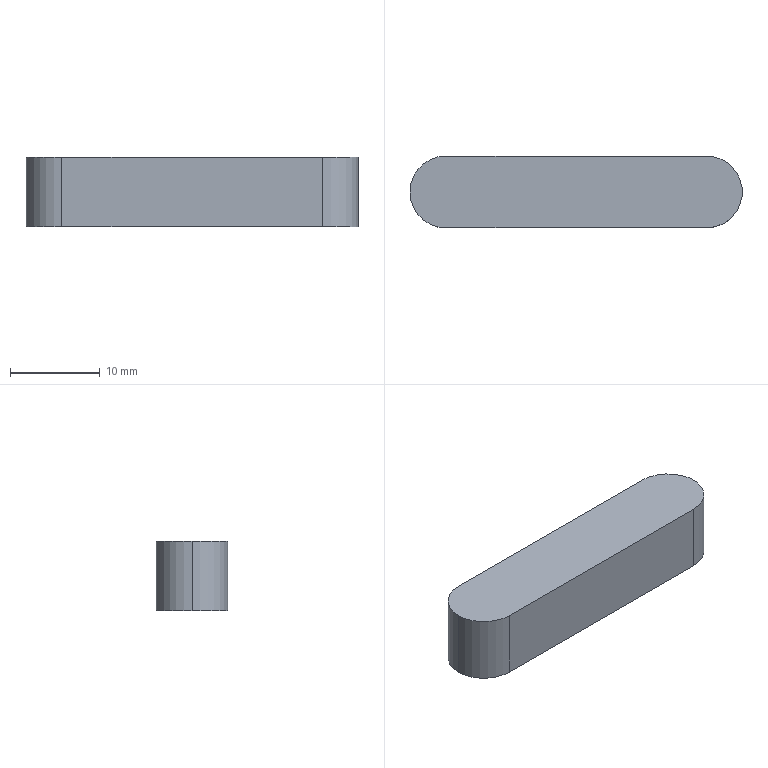Part | STEP file | Keyway 8x38V11_Default<Machined> | 1 solid | 7 faces | box 37 x 8 x 7.7 mm | volume 2173 mm3 | plane 4 | cylinder 3 | commonest cylinder face diameters 8 x3
STEP:
#1=CARTESIAN_POINT('',(0.,0.,0.));
#2=DIRECTION('',(0.,0.,1.));
#3=DIRECTION('',(1.,0.,0.));
#4=AXIS2_PLACEMENT_3D('',#1,#2,#3);
#5=CARTESIAN_POINT('',(-33.,0.,7.7));
#6=VERTEX_POINT('',#5);
#7=CARTESIAN_POINT('',(-29.,-4.,7.7));
#8=VERTEX_POINT('',#7);
#9=CARTESIAN_POINT('',(-29.,0.,7.7));
#10=DIRECTION('',(0.,0.,1.));
#11=DIRECTION('',(1.,0.,0.));
#12=AXIS2_PLACEMENT_3D('',#9,#10,#11);
#13=CIRCLE('',#12,4.);
#14=CARTESIAN_POINT('',(-29.,0.,7.7));
#15=DIRECTION('',(0.,0.,-1.));
#16=DIRECTION('',(-1.,0.,0.));
#17=AXIS2_PLACEMENT_3D('',#14,#15,#16);
#18=CYLINDRICAL_SURFACE('',#17,4.);
#19=CARTESIAN_POINT('',(9.425,0.));
#20=DIRECTION('',(-1.,0.));
#21=VECTOR('',#20,1.);
#22=LINE('',#19,#21);
#23=(GEOMETRIC_REPRESENTATION_CONTEXT(2)PARAMETRIC_REPRESENTATION_CONTEXT()REPRESENTATION_CONTEXT('',''));
#24=DEFINITIONAL_REPRESENTATION('',(#22),#23);
#25=PCURVE('',#18,#24);
#26=CARTESIAN_POINT('',(0.,0.,7.7));
#27=DIRECTION('',(0.,0.,1.));
#28=DIRECTION('',(1.,0.,0.));
#29=AXIS2_PLACEMENT_3D('',#26,#27,#28);
#30=PLANE('',#29);
#31=CARTESIAN_POINT('',(-29.,0.));
#32=DIRECTION('',(1.,0.));
#33=AXIS2_PLACEMENT_2D('',#31,#32);
#34=CIRCLE('',#33,4.);
#35=(GEOMETRIC_REPRESENTATION_CONTEXT(2)PARAMETRIC_REPRESENTATION_CONTEXT()REPRESENTATION_CONTEXT('',''));
#36=DEFINITIONAL_REPRESENTATION('',(#34),#35);
#37=PCURVE('',#30,#36);
#38=SURFACE_CURVE('',#13,(#25,#37),.PCURVE_S1.);
#39=EDGE_CURVE('',#6,#8,#38,.T.);
#40=ORIENTED_EDGE('',*,*,#39,.F.);
#41=CARTESIAN_POINT('',(-33.,0.,0.));
#42=VERTEX_POINT('',#41);
#43=CARTESIAN_POINT('',(-33.,0.,7.7));
#44=DIRECTION('',(0.,0.,-1.));
#45=VECTOR('',#44,1.);
#46=LINE('',#43,#45);
#47=CARTESIAN_POINT('',(6.283,0.));
#48=DIRECTION('',(0.,1.));
#49=VECTOR('',#48,1.);
#50=LINE('',#47,#49);
#51=(GEOMETRIC_REPRESENTATION_CONTEXT(2)PARAMETRIC_REPRESENTATION_CONTEXT()REPRESENTATION_CONTEXT('',''));
#52=DEFINITIONAL_REPRESENTATION('',(#50),#51);
#53=PCURVE('',#18,#52);
#54=CARTESIAN_POINT('',(-29.,0.,7.7));
#55=DIRECTION('',(0.,0.,-1.));
#56=DIRECTION('',(-1.,0.,0.));
#57=AXIS2_PLACEMENT_3D('',#54,#55,#56);
#58=CYLINDRICAL_SURFACE('',#57,4.);
#59=CARTESIAN_POINT('',(0.,0.));
#60=DIRECTION('',(0.,1.));
#61=VECTOR('',#60,1.);
#62=LINE('',#59,#61);
#63=(GEOMETRIC_REPRESENTATION_CONTEXT(2)PARAMETRIC_REPRESENTATION_CONTEXT()REPRESENTATION_CONTEXT('',''));
#64=DEFINITIONAL_REPRESENTATION('',(#62),#63);
#65=PCURVE('',#58,#64);
#66=SURFACE_CURVE('',#46,(#53,#65),.PCURVE_S1.);
#67=EDGE_CURVE('',#6,#42,#66,.T.);
#68=ORIENTED_EDGE('',*,*,#67,.T.);
#69=CARTESIAN_POINT('',(-29.,-4.,0.));
#70=VERTEX_POINT('',#69);
#71=CARTESIAN_POINT('',(-29.,0.,0.));
#72=DIRECTION('',(0.,0.,1.));
#73=DIRECTION('',(1.,0.,0.));
#74=AXIS2_PLACEMENT_3D('',#71,#72,#73);
#75=CIRCLE('',#74,4.);
#76=CARTESIAN_POINT('',(9.425,7.7));
#77=DIRECTION('',(-1.,0.));
#78=VECTOR('',#77,1.);
#79=LINE('',#76,#78);
#80=(GEOMETRIC_REPRESENTATION_CONTEXT(2)PARAMETRIC_REPRESENTATION_CONTEXT()REPRESENTATION_CONTEXT('',''));
#81=DEFINITIONAL_REPRESENTATION('',(#79),#80);
#82=PCURVE('',#18,#81);
#83=CARTESIAN_POINT('',(0.,0.,0.));
#84=DIRECTION('',(0.,0.,1.));
#85=DIRECTION('',(1.,0.,0.));
#86=AXIS2_PLACEMENT_3D('',#83,#84,#85);
#87=PLANE('',#86);
#88=CARTESIAN_POINT('',(-29.,0.));
#89=DIRECTION('',(1.,0.));
#90=AXIS2_PLACEMENT_2D('',#88,#89);
#91=CIRCLE('',#90,4.);
#92=(GEOMETRIC_REPRESENTATION_CONTEXT(2)PARAMETRIC_REPRESENTATION_CONTEXT()REPRESENTATION_CONTEXT('',''));
#93=DEFINITIONAL_REPRESENTATION('',(#91),#92);
#94=PCURVE('',#87,#93);
#95=SURFACE_CURVE('',#75,(#82,#94),.PCURVE_S1.);
#96=EDGE_CURVE('',#42,#70,#95,.T.);
#97=ORIENTED_EDGE('',*,*,#96,.T.);
#98=CARTESIAN_POINT('',(-29.,-4.,7.7));
#99=DIRECTION('',(0.,0.,-1.));
#100=VECTOR('',#99,1.);
#101=LINE('',#98,#100);
#102=CARTESIAN_POINT('',(4.712,0.));
#103=DIRECTION('',(0.,1.));
#104=VECTOR('',#103,1.);
#105=LINE('',#102,#104);
#106=(GEOMETRIC_REPRESENTATION_CONTEXT(2)PARAMETRIC_REPRESENTATION_CONTEXT()REPRESENTATION_CONTEXT('',''));
#107=DEFINITIONAL_REPRESENTATION('',(#105),#106);
#108=PCURVE('',#18,#107);
#109=CARTESIAN_POINT('',(0.,-4.,7.7));
#110=DIRECTION('',(0.,1.,0.));
#111=DIRECTION('',(-1.,0.,0.));
#112=AXIS2_PLACEMENT_3D('',#109,#110,#111);
#113=PLANE('',#112);
#114=CARTESIAN_POINT('',(29.,0.));
#115=DIRECTION('',(0.,-1.));
#116=VECTOR('',#115,1.);
#117=LINE('',#114,#116);
#118=(GEOMETRIC_REPRESENTATION_CONTEXT(2)PARAMETRIC_REPRESENTATION_CONTEXT()REPRESENTATION_CONTEXT('',''));
#119=DEFINITIONAL_REPRESENTATION('',(#117),#118);
#120=PCURVE('',#113,#119);
#121=SURFACE_CURVE('',#101,(#108,#120),.PCURVE_S1.);
#122=EDGE_CURVE('',#8,#70,#121,.T.);
#123=ORIENTED_EDGE('',*,*,#122,.F.);
#124=EDGE_LOOP('',(#40,#68,#97,#123));
#125=FACE_BOUND('',#124,.T.);
#126=ADVANCED_FACE('',(#125),#18,.T.);
#127=CARTESIAN_POINT('',(0.,-4.,0.));
#128=VERTEX_POINT('',#127);
#129=CARTESIAN_POINT('',(0.,4.,0.));
#130=VERTEX_POINT('',#129);
#131=CARTESIAN_POINT('',(0.,0.,0.));
#132=DIRECTION('',(0.,0.,1.));
#133=DIRECTION('',(1.,0.,0.));
#134=AXIS2_PLACEMENT_3D('',#131,#132,#133);
#135=CIRCLE('',#134,4.);
#136=CARTESIAN_POINT('',(0.,0.,7.7));
#137=DIRECTION('',(0.,0.,-1.));
#138=DIRECTION('',(-1.,0.,0.));
#139=AXIS2_PLACEMENT_3D('',#136,#137,#138);
#140=CYLINDRICAL_SURFACE('',#139,4.);
#141=CARTESIAN_POINT('',(9.425,7.7));
#142=DIRECTION('',(-1.,0.));
#143=VECTOR('',#142,1.);
#144=LINE('',#141,#143);
#145=(GEOMETRIC_REPRESENTATION_CONTEXT(2)PARAMETRIC_REPRESENTATION_CONTEXT()REPRESENTATION_CONTEXT('',''));
#146=DEFINITIONAL_REPRESENTATION('',(#144),#145);
#147=PCURVE('',#140,#146);
#148=CARTESIAN_POINT('',(0.,0.));
#149=DIRECTION('',(1.,0.));
#150=AXIS2_PLACEMENT_2D('',#148,#149);
#151=CIRCLE('',#150,4.);
#152=(GEOMETRIC_REPRESENTATION_CONTEXT(2)PARAMETRIC_REPRESENTATION_CONTEXT()REPRESENTATION_CONTEXT('',''));
#153=DEFINITIONAL_REPRESENTATION('',(#151),#152);
#154=PCURVE('',#87,#153);
#155=SURFACE_CURVE('',#135,(#147,#154),.PCURVE_S1.);
#156=EDGE_CURVE('',#128,#130,#155,.T.);
#157=ORIENTED_EDGE('',*,*,#156,.T.);
#158=CARTESIAN_POINT('',(0.,4.,7.7));
#159=VERTEX_POINT('',#158);
#160=CARTESIAN_POINT('',(0.,4.,7.7));
#161=DIRECTION('',(0.,0.,-1.));
#162=VECTOR('',#161,1.);
#163=LINE('',#160,#162);
#164=CARTESIAN_POINT('',(1.571,0.));
#165=DIRECTION('',(0.,1.));
#166=VECTOR('',#165,1.);
#167=LINE('',#164,#166);
#168=(GEOMETRIC_REPRESENTATION_CONTEXT(2)PARAMETRIC_REPRESENTATION_CONTEXT()REPRESENTATION_CONTEXT('',''));
#169=DEFINITIONAL_REPRESENTATION('',(#167),#168);
#170=PCURVE('',#140,#169);
#171=CARTESIAN_POINT('',(0.,4.,7.7));
#172=DIRECTION('',(0.,-1.,0.));
#173=DIRECTION('',(1.,0.,0.));
#174=AXIS2_PLACEMENT_3D('',#171,#172,#173);
#175=PLANE('',#174);
#176=CARTESIAN_POINT('',(0.,0.));
#177=DIRECTION('',(0.,-1.));
#178=VECTOR('',#177,1.);
#179=LINE('',#176,#178);
#180=(GEOMETRIC_REPRESENTATION_CONTEXT(2)PARAMETRIC_REPRESENTATION_CONTEXT()REPRESENTATION_CONTEXT('',''));
#181=DEFINITIONAL_REPRESENTATION('',(#179),#180);
#182=PCURVE('',#175,#181);
#183=SURFACE_CURVE('',#163,(#170,#182),.PCURVE_S1.);
#184=EDGE_CURVE('',#159,#130,#183,.T.);
#185=ORIENTED_EDGE('',*,*,#184,.F.);
#186=CARTESIAN_POINT('',(0.,-4.,7.7));
#187=VERTEX_POINT('',#186);
#188=CARTESIAN_POINT('',(0.,0.,7.7));
#189=DIRECTION('',(0.,0.,1.));
#190=DIRECTION('',(1.,0.,0.));
#191=AXIS2_PLACEMENT_3D('',#188,#189,#190);
#192=CIRCLE('',#191,4.);
#193=CARTESIAN_POINT('',(9.425,0.));
#194=DIRECTION('',(-1.,0.));
#195=VECTOR('',#194,1.);
#196=LINE('',#193,#195);
#197=(GEOMETRIC_REPRESENTATION_CONTEXT(2)PARAMETRIC_REPRESENTATION_CONTEXT()REPRESENTATION_CONTEXT('',''));
#198=DEFINITIONAL_REPRESENTATION('',(#196),#197);
#199=PCURVE('',#140,#198);
#200=CARTESIAN_POINT('',(0.,0.));
#201=DIRECTION('',(1.,0.));
#202=AXIS2_PLACEMENT_2D('',#200,#201);
#203=CIRCLE('',#202,4.);
#204=(GEOMETRIC_REPRESENTATION_CONTEXT(2)PARAMETRIC_REPRESENTATION_CONTEXT()REPRESENTATION_CONTEXT('',''));
#205=DEFINITIONAL_REPRESENTATION('',(#203),#204);
#206=PCURVE('',#30,#205);
#207=SURFACE_CURVE('',#192,(#199,#206),.PCURVE_S1.);
#208=EDGE_CURVE('',#187,#159,#207,.T.);
#209=ORIENTED_EDGE('',*,*,#208,.F.);
#210=CARTESIAN_POINT('',(0.,-4.,7.7));
#211=DIRECTION('',(0.,0.,-1.));
#212=VECTOR('',#211,1.);
#213=LINE('',#210,#212);
#214=CARTESIAN_POINT('',(4.712,0.));
#215=DIRECTION('',(0.,1.));
#216=VECTOR('',#215,1.);
#217=LINE('',#214,#216);
#218=(GEOMETRIC_REPRESENTATION_CONTEXT(2)PARAMETRIC_REPRESENTATION_CONTEXT()REPRESENTATION_CONTEXT('',''));
#219=DEFINITIONAL_REPRESENTATION('',(#217),#218);
#220=PCURVE('',#140,#219);
#221=CARTESIAN_POINT('',(0.,0.));
#222=DIRECTION('',(0.,-1.));
#223=VECTOR('',#222,1.);
#224=LINE('',#221,#223);
#225=(GEOMETRIC_REPRESENTATION_CONTEXT(2)PARAMETRIC_REPRESENTATION_CONTEXT()REPRESENTATION_CONTEXT('',''));
#226=DEFINITIONAL_REPRESENTATION('',(#224),#225);
#227=PCURVE('',#113,#226);
#228=SURFACE_CURVE('',#213,(#220,#227),.PCURVE_S1.);
#229=EDGE_CURVE('',#187,#128,#228,.T.);
#230=ORIENTED_EDGE('',*,*,#229,.T.);
#231=EDGE_LOOP('',(#157,#185,#209,#230));
#232=FACE_BOUND('',#231,.T.);
#233=ADVANCED_FACE('',(#232),#140,.T.);
#234=CARTESIAN_POINT('',(-29.,4.,0.));
#235=VERTEX_POINT('',#234);
#236=CARTESIAN_POINT('',(0.,4.,0.));
#237=DIRECTION('',(-1.,0.,0.));
#238=VECTOR('',#237,1.);
#239=LINE('',#236,#238);
#240=CARTESIAN_POINT('',(0.,-7.7));
#241=DIRECTION('',(-1.,0.));
#242=VECTOR('',#241,1.);
#243=LINE('',#240,#242);
#244=(GEOMETRIC_REPRESENTATION_CONTEXT(2)PARAMETRIC_REPRESENTATION_CONTEXT()REPRESENTATION_CONTEXT('',''));
#245=DEFINITIONAL_REPRESENTATION('',(#243),#244);
#246=PCURVE('',#175,#245);
#247=CARTESIAN_POINT('',(0.,4.));
#248=DIRECTION('',(-1.,0.));
#249=VECTOR('',#248,1.);
#250=LINE('',#247,#249);
#251=(GEOMETRIC_REPRESENTATION_CONTEXT(2)PARAMETRIC_REPRESENTATION_CONTEXT()REPRESENTATION_CONTEXT('',''));
#252=DEFINITIONAL_REPRESENTATION('',(#250),#251);
#253=PCURVE('',#87,#252);
#254=SURFACE_CURVE('',#239,(#246,#253),.PCURVE_S1.);
#255=EDGE_CURVE('',#130,#235,#254,.T.);
#256=ORIENTED_EDGE('',*,*,#255,.T.);
#257=CARTESIAN_POINT('',(-29.,4.,7.7));
#258=VERTEX_POINT('',#257);
#259=CARTESIAN_POINT('',(-29.,4.,7.7));
#260=DIRECTION('',(0.,0.,-1.));
#261=VECTOR('',#260,1.);
#262=LINE('',#259,#261);
#263=CARTESIAN_POINT('',(-29.,0.));
#264=DIRECTION('',(0.,-1.));
#265=VECTOR('',#264,1.);
#266=LINE('',#263,#265);
#267=(GEOMETRIC_REPRESENTATION_CONTEXT(2)PARAMETRIC_REPRESENTATION_CONTEXT()REPRESENTATION_CONTEXT('',''));
#268=DEFINITIONAL_REPRESENTATION('',(#266),#267);
#269=PCURVE('',#175,#268);
#270=CARTESIAN_POINT('',(1.571,0.));
#271=DIRECTION('',(0.,1.));
#272=VECTOR('',#271,1.);
#273=LINE('',#270,#272);
#274=(GEOMETRIC_REPRESENTATION_CONTEXT(2)PARAMETRIC_REPRESENTATION_CONTEXT()REPRESENTATION_CONTEXT('',''));
#275=DEFINITIONAL_REPRESENTATION('',(#273),#274);
#276=PCURVE('',#58,#275);
#277=SURFACE_CURVE('',#262,(#269,#276),.PCURVE_S1.);
#278=EDGE_CURVE('',#258,#235,#277,.T.);
#279=ORIENTED_EDGE('',*,*,#278,.F.);
#280=CARTESIAN_POINT('',(0.,4.,7.7));
#281=DIRECTION('',(-1.,0.,0.));
#282=VECTOR('',#281,1.);
#283=LINE('',#280,#282);
#284=CARTESIAN_POINT('',(0.,0.));
#285=DIRECTION('',(-1.,0.));
#286=VECTOR('',#285,1.);
#287=LINE('',#284,#286);
#288=(GEOMETRIC_REPRESENTATION_CONTEXT(2)PARAMETRIC_REPRESENTATION_CONTEXT()REPRESENTATION_CONTEXT('',''));
#289=DEFINITIONAL_REPRESENTATION('',(#287),#288);
#290=PCURVE('',#175,#289);
#291=CARTESIAN_POINT('',(0.,4.));
#292=DIRECTION('',(-1.,0.));
#293=VECTOR('',#292,1.);
#294=LINE('',#291,#293);
#295=(GEOMETRIC_REPRESENTATION_CONTEXT(2)PARAMETRIC_REPRESENTATION_CONTEXT()REPRESENTATION_CONTEXT('',''));
#296=DEFINITIONAL_REPRESENTATION('',(#294),#295);
#297=PCURVE('',#30,#296);
#298=SURFACE_CURVE('',#283,(#290,#297),.PCURVE_S1.);
#299=EDGE_CURVE('',#159,#258,#298,.T.);
#300=ORIENTED_EDGE('',*,*,#299,.F.);
#301=ORIENTED_EDGE('',*,*,#184,.T.);
#302=EDGE_LOOP('',(#256,#279,#300,#301));
#303=FACE_BOUND('',#302,.T.);
#304=ADVANCED_FACE('',(#303),#175,.F.);
#305=ORIENTED_EDGE('',*,*,#67,.F.);
#306=CARTESIAN_POINT('',(-29.,0.,7.7));
#307=DIRECTION('',(0.,0.,1.));
#308=DIRECTION('',(1.,0.,0.));
#309=AXIS2_PLACEMENT_3D('',#306,#307,#308);
#310=CIRCLE('',#309,4.);
#311=CARTESIAN_POINT('',(3.142,0.));
#312=DIRECTION('',(-1.,0.));
#313=VECTOR('',#312,1.);
#314=LINE('',#311,#313);
#315=(GEOMETRIC_REPRESENTATION_CONTEXT(2)PARAMETRIC_REPRESENTATION_CONTEXT()REPRESENTATION_CONTEXT('',''));
#316=DEFINITIONAL_REPRESENTATION('',(#314),#315);
#317=PCURVE('',#58,#316);
#318=CARTESIAN_POINT('',(-29.,0.));
#319=DIRECTION('',(1.,0.));
#320=AXIS2_PLACEMENT_2D('',#318,#319);
#321=CIRCLE('',#320,4.);
#322=(GEOMETRIC_REPRESENTATION_CONTEXT(2)PARAMETRIC_REPRESENTATION_CONTEXT()REPRESENTATION_CONTEXT('',''));
#323=DEFINITIONAL_REPRESENTATION('',(#321),#322);
#324=PCURVE('',#30,#323);
#325=SURFACE_CURVE('',#310,(#317,#324),.PCURVE_S1.);
#326=EDGE_CURVE('',#258,#6,#325,.T.);
#327=ORIENTED_EDGE('',*,*,#326,.F.);
#328=ORIENTED_EDGE('',*,*,#278,.T.);
#329=CARTESIAN_POINT('',(-29.,0.,0.));
#330=DIRECTION('',(0.,0.,1.));
#331=DIRECTION('',(1.,0.,0.));
#332=AXIS2_PLACEMENT_3D('',#329,#330,#331);
#333=CIRCLE('',#332,4.);
#334=CARTESIAN_POINT('',(3.142,7.7));
#335=DIRECTION('',(-1.,0.));
#336=VECTOR('',#335,1.);
#337=LINE('',#334,#336);
#338=(GEOMETRIC_REPRESENTATION_CONTEXT(2)PARAMETRIC_REPRESENTATION_CONTEXT()REPRESENTATION_CONTEXT('',''));
#339=DEFINITIONAL_REPRESENTATION('',(#337),#338);
#340=PCURVE('',#58,#339);
#341=CARTESIAN_POINT('',(-29.,0.));
#342=DIRECTION('',(1.,0.));
#343=AXIS2_PLACEMENT_2D('',#341,#342);
#344=CIRCLE('',#343,4.);
#345=(GEOMETRIC_REPRESENTATION_CONTEXT(2)PARAMETRIC_REPRESENTATION_CONTEXT()REPRESENTATION_CONTEXT('',''));
#346=DEFINITIONAL_REPRESENTATION('',(#344),#345);
#347=PCURVE('',#87,#346);
#348=SURFACE_CURVE('',#333,(#340,#347),.PCURVE_S1.);
#349=EDGE_CURVE('',#235,#42,#348,.T.);
#350=ORIENTED_EDGE('',*,*,#349,.T.);
#351=EDGE_LOOP('',(#305,#327,#328,#350));
#352=FACE_BOUND('',#351,.T.);
#353=ADVANCED_FACE('',(#352),#58,.T.);
#354=CARTESIAN_POINT('',(0.,-4.,0.));
#355=DIRECTION('',(1.,0.,0.));
#356=VECTOR('',#355,1.);
#357=LINE('',#354,#356);
#358=CARTESIAN_POINT('',(0.,-7.7));
#359=DIRECTION('',(-1.,0.));
#360=VECTOR('',#359,1.);
#361=LINE('',#358,#360);
#362=(GEOMETRIC_REPRESENTATION_CONTEXT(2)PARAMETRIC_REPRESENTATION_CONTEXT()REPRESENTATION_CONTEXT('',''));
#363=DEFINITIONAL_REPRESENTATION('',(#361),#362);
#364=PCURVE('',#113,#363);
#365=CARTESIAN_POINT('',(0.,-4.));
#366=DIRECTION('',(1.,0.));
#367=VECTOR('',#366,1.);
#368=LINE('',#365,#367);
#369=(GEOMETRIC_REPRESENTATION_CONTEXT(2)PARAMETRIC_REPRESENTATION_CONTEXT()REPRESENTATION_CONTEXT('',''));
#370=DEFINITIONAL_REPRESENTATION('',(#368),#369);
#371=PCURVE('',#87,#370);
#372=SURFACE_CURVE('',#357,(#364,#371),.PCURVE_S1.);
#373=EDGE_CURVE('',#70,#128,#372,.T.);
#374=ORIENTED_EDGE('',*,*,#373,.T.);
#375=ORIENTED_EDGE('',*,*,#229,.F.);
#376=CARTESIAN_POINT('',(0.,-4.,7.7));
#377=DIRECTION('',(1.,0.,0.));
#378=VECTOR('',#377,1.);
#379=LINE('',#376,#378);
#380=CARTESIAN_POINT('',(0.,0.));
#381=DIRECTION('',(-1.,0.));
#382=VECTOR('',#381,1.);
#383=LINE('',#380,#382);
#384=(GEOMETRIC_REPRESENTATION_CONTEXT(2)PARAMETRIC_REPRESENTATION_CONTEXT()REPRESENTATION_CONTEXT('',''));
#385=DEFINITIONAL_REPRESENTATION('',(#383),#384);
#386=PCURVE('',#113,#385);
#387=CARTESIAN_POINT('',(0.,-4.));
#388=DIRECTION('',(1.,0.));
#389=VECTOR('',#388,1.);
#390=LINE('',#387,#389);
#391=(GEOMETRIC_REPRESENTATION_CONTEXT(2)PARAMETRIC_REPRESENTATION_CONTEXT()REPRESENTATION_CONTEXT('',''));
#392=DEFINITIONAL_REPRESENTATION('',(#390),#391);
#393=PCURVE('',#30,#392);
#394=SURFACE_CURVE('',#379,(#386,#393),.PCURVE_S1.);
#395=EDGE_CURVE('',#8,#187,#394,.T.);
#396=ORIENTED_EDGE('',*,*,#395,.F.);
#397=ORIENTED_EDGE('',*,*,#122,.T.);
#398=EDGE_LOOP('',(#374,#375,#396,#397));
#399=FACE_BOUND('',#398,.T.);
#400=ADVANCED_FACE('',(#399),#113,.F.);
#401=ORIENTED_EDGE('',*,*,#208,.T.);
#402=ORIENTED_EDGE('',*,*,#299,.T.);
#403=ORIENTED_EDGE('',*,*,#326,.T.);
#404=ORIENTED_EDGE('',*,*,#39,.T.);
#405=ORIENTED_EDGE('',*,*,#395,.T.);
#406=EDGE_LOOP('',(#401,#402,#403,#404,#405));
#407=FACE_BOUND('',#406,.T.);
#408=ADVANCED_FACE('',(#407),#30,.T.);
#409=ORIENTED_EDGE('',*,*,#156,.F.);
#410=ORIENTED_EDGE('',*,*,#373,.F.);
#411=ORIENTED_EDGE('',*,*,#96,.F.);
#412=ORIENTED_EDGE('',*,*,#349,.F.);
#413=ORIENTED_EDGE('',*,*,#255,.F.);
#414=EDGE_LOOP('',(#409,#410,#411,#412,#413));
#415=FACE_BOUND('',#414,.T.);
#416=ADVANCED_FACE('',(#415),#87,.F.);
#417=CLOSED_SHELL('',(#126,#233,#304,#353,#400,#408,#416));
#418=MANIFOLD_SOLID_BREP('',#417);
#419=(LENGTH_UNIT()NAMED_UNIT(*)SI_UNIT(.MILLI.,.METRE.));
#420=UNCERTAINTY_MEASURE_WITH_UNIT(LENGTH_MEASURE(0.0000001),#419,'','');
#421=(NAMED_UNIT(*)PLANE_ANGLE_UNIT()SI_UNIT($,.RADIAN.));
#422=(NAMED_UNIT(*)SI_UNIT($,.STERADIAN.)SOLID_ANGLE_UNIT());
#423=(GEOMETRIC_REPRESENTATION_CONTEXT(3)GLOBAL_UNCERTAINTY_ASSIGNED_CONTEXT((#420))GLOBAL_UNIT_ASSIGNED_CONTEXT((#419,#421,#422))REPRESENTATION_CONTEXT('',''));
#424=ADVANCED_BREP_SHAPE_REPRESENTATION('',(#4,#418),#423);